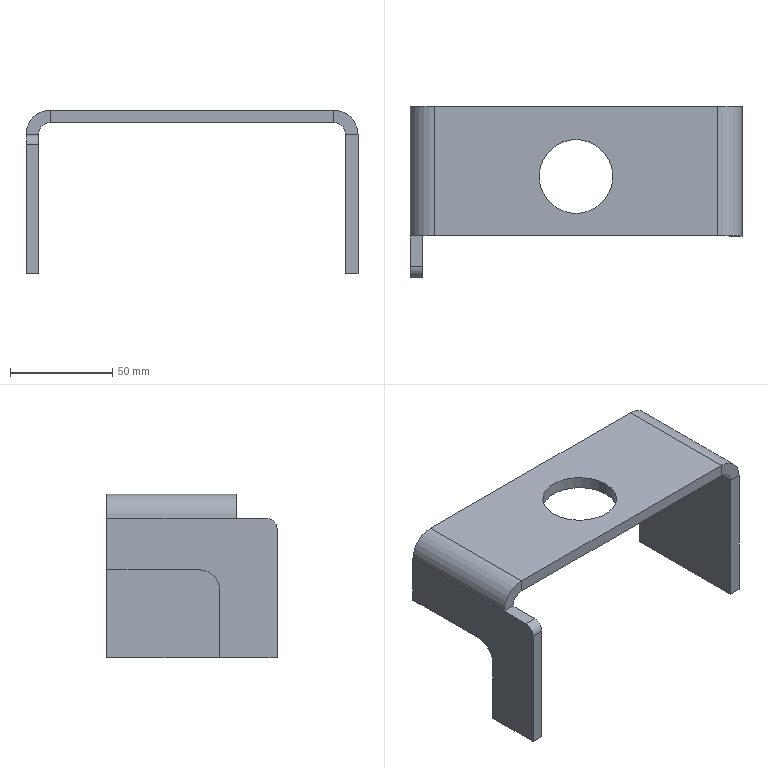Part | SolidWorks | features ICE 3, Fillet 2, FlatPattern 1, SMBaseFlange 1, SheetMetal 1 | 1 solid | 29 faces | box 162 x 83 x 80 mm | volume 102219 mm3 | plane 21 | cylinder 8 | commonest cylinder face diameters 12 x2 24 x2 36 x2 10 x1 20 x1
STEP:
#1=CARTESIAN_POINT('',(63.,49.,-6.));
#2=VERTEX_POINT('',#1);
#3=CARTESIAN_POINT('',(99.,49.,-6.));
#4=VERTEX_POINT('',#3);
#5=CARTESIAN_POINT('',(81.,49.,-6.));
#6=DIRECTION('',(0.,0.,1.));
#7=DIRECTION('',(1.,0.,0.));
#8=AXIS2_PLACEMENT_3D('',#5,#6,#7);
#9=CIRCLE('',#8,18.);
#10=EDGE_CURVE('',#2,#4,#9,.T.);
#11=ORIENTED_EDGE('',*,*,#10,.F.);
#12=CARTESIAN_POINT('',(63.,49.,0.));
#13=VERTEX_POINT('',#12);
#14=CARTESIAN_POINT('',(63.,49.,-6.));
#15=DIRECTION('',(0.,0.,1.));
#16=VECTOR('',#15,1000.);
#17=LINE('',#14,#16);
#18=EDGE_CURVE('',#2,#13,#17,.T.);
#19=ORIENTED_EDGE('',*,*,#18,.T.);
#20=CARTESIAN_POINT('',(99.,49.,0.));
#21=VERTEX_POINT('',#20);
#22=CARTESIAN_POINT('',(81.,49.,0.));
#23=DIRECTION('',(0.,0.,1.));
#24=DIRECTION('',(1.,0.,0.));
#25=AXIS2_PLACEMENT_3D('',#22,#23,#24);
#26=CIRCLE('',#25,18.);
#27=EDGE_CURVE('',#13,#21,#26,.T.);
#28=ORIENTED_EDGE('',*,*,#27,.T.);
#29=CARTESIAN_POINT('',(99.,49.,-6.));
#30=DIRECTION('',(0.,0.,1.));
#31=VECTOR('',#30,1000.);
#32=LINE('',#29,#31);
#33=EDGE_CURVE('',#4,#21,#32,.T.);
#34=ORIENTED_EDGE('',*,*,#33,.F.);
#35=EDGE_LOOP('',(#11,#19,#28,#34));
#36=FACE_OUTER_BOUND('',#35,.T.);
#37=CARTESIAN_POINT('',(81.,49.,-6.));
#38=DIRECTION('',(0.,0.,1.));
#39=DIRECTION('',(1.,0.,0.));
#40=AXIS2_PLACEMENT_3D('',#37,#38,#39);
#41=CYLINDRICAL_SURFACE('',#40,18.);
#42=ADVANCED_FACE('',(#36),#41,.F.);
#43=CARTESIAN_POINT('',(162.,20.,-12.));
#44=VERTEX_POINT('',#43);
#45=CARTESIAN_POINT('',(162.,20.,-80.));
#46=VERTEX_POINT('',#45);
#47=CARTESIAN_POINT('',(162.,20.,0.));
#48=DIRECTION('',(0.,0.,-1.));
#49=VECTOR('',#48,1000.);
#50=LINE('',#47,#49);
#51=EDGE_CURVE('',#44,#46,#50,.T.);
#52=ORIENTED_EDGE('',*,*,#51,.T.);
#53=CARTESIAN_POINT('',(162.,83.,-80.));
#54=VERTEX_POINT('',#53);
#55=CARTESIAN_POINT('',(162.,83.,-80.));
#56=DIRECTION('',(0.,-1.,0.));
#57=VECTOR('',#56,1000.);
#58=LINE('',#55,#57);
#59=EDGE_CURVE('',#54,#46,#58,.T.);
#60=ORIENTED_EDGE('',*,*,#59,.F.);
#61=CARTESIAN_POINT('',(162.,83.,-12.));
#62=VERTEX_POINT('',#61);
#63=CARTESIAN_POINT('',(162.,83.,0.));
#64=DIRECTION('',(0.,0.,-1.));
#65=VECTOR('',#64,1000.);
#66=LINE('',#63,#65);
#67=EDGE_CURVE('',#62,#54,#66,.T.);
#68=ORIENTED_EDGE('',*,*,#67,.F.);
#69=CARTESIAN_POINT('',(162.,83.,-12.));
#70=DIRECTION('',(0.,-1.,0.));
#71=VECTOR('',#70,1000.);
#72=LINE('',#69,#71);
#73=EDGE_CURVE('',#62,#44,#72,.T.);
#74=ORIENTED_EDGE('',*,*,#73,.T.);
#75=EDGE_LOOP('',(#52,#60,#68,#74));
#76=FACE_OUTER_BOUND('',#75,.T.);
#77=CARTESIAN_POINT('',(162.,83.,0.));
#78=DIRECTION('',(-1.,0.,0.));
#79=DIRECTION('',(0.,0.,1.));
#80=AXIS2_PLACEMENT_3D('',#77,#78,#79);
#81=PLANE('',#80);
#82=ADVANCED_FACE('',(#76),#81,.F.);
#83=ORIENTED_EDGE('',*,*,#59,.T.);
#84=CARTESIAN_POINT('',(156.,20.,-80.));
#85=VERTEX_POINT('',#84);
#86=CARTESIAN_POINT('',(156.,20.,-80.));
#87=DIRECTION('',(1.,0.,0.));
#88=VECTOR('',#87,1000.);
#89=LINE('',#86,#88);
#90=EDGE_CURVE('',#85,#46,#89,.T.);
#91=ORIENTED_EDGE('',*,*,#90,.F.);
#92=CARTESIAN_POINT('',(156.,83.,-80.));
#93=VERTEX_POINT('',#92);
#94=CARTESIAN_POINT('',(156.,83.,-80.));
#95=DIRECTION('',(0.,-1.,0.));
#96=VECTOR('',#95,1000.);
#97=LINE('',#94,#96);
#98=EDGE_CURVE('',#93,#85,#97,.T.);
#99=ORIENTED_EDGE('',*,*,#98,.F.);
#100=CARTESIAN_POINT('',(156.,83.,-80.));
#101=DIRECTION('',(1.,0.,0.));
#102=VECTOR('',#101,1000.);
#103=LINE('',#100,#102);
#104=EDGE_CURVE('',#93,#54,#103,.T.);
#105=ORIENTED_EDGE('',*,*,#104,.T.);
#106=EDGE_LOOP('',(#83,#91,#99,#105));
#107=FACE_OUTER_BOUND('',#106,.T.);
#108=CARTESIAN_POINT('',(156.,83.,-80.));
#109=DIRECTION('',(0.,0.,-1.));
#110=DIRECTION('',(-1.,0.,0.));
#111=AXIS2_PLACEMENT_3D('',#108,#109,#110);
#112=PLANE('',#111);
#113=ADVANCED_FACE('',(#107),#112,.T.);
#114=ORIENTED_EDGE('',*,*,#98,.T.);
#115=CARTESIAN_POINT('',(156.,20.,-12.));
#116=VERTEX_POINT('',#115);
#117=CARTESIAN_POINT('',(156.,20.,0.));
#118=DIRECTION('',(0.,0.,-1.));
#119=VECTOR('',#118,1000.);
#120=LINE('',#117,#119);
#121=EDGE_CURVE('',#116,#85,#120,.T.);
#122=ORIENTED_EDGE('',*,*,#121,.F.);
#123=CARTESIAN_POINT('',(156.,83.,-12.));
#124=VERTEX_POINT('',#123);
#125=CARTESIAN_POINT('',(156.,83.,-12.));
#126=DIRECTION('',(0.,-1.,0.));
#127=VECTOR('',#126,1000.);
#128=LINE('',#125,#127);
#129=EDGE_CURVE('',#124,#116,#128,.T.);
#130=ORIENTED_EDGE('',*,*,#129,.F.);
#131=CARTESIAN_POINT('',(156.,83.,0.));
#132=DIRECTION('',(0.,0.,-1.));
#133=VECTOR('',#132,1000.);
#134=LINE('',#131,#133);
#135=EDGE_CURVE('',#124,#93,#134,.T.);
#136=ORIENTED_EDGE('',*,*,#135,.T.);
#137=EDGE_LOOP('',(#114,#122,#130,#136));
#138=FACE_OUTER_BOUND('',#137,.T.);
#139=CARTESIAN_POINT('',(156.,83.,0.));
#140=DIRECTION('',(-1.,0.,0.));
#141=DIRECTION('',(0.,0.,1.));
#142=AXIS2_PLACEMENT_3D('',#139,#140,#141);
#143=PLANE('',#142);
#144=ADVANCED_FACE('',(#138),#143,.T.);
#145=ORIENTED_EDGE('',*,*,#129,.T.);
#146=CARTESIAN_POINT('',(150.,20.,-6.));
#147=VERTEX_POINT('',#146);
#148=CARTESIAN_POINT('',(150.,20.,-12.));
#149=DIRECTION('',(0.,1.,0.));
#150=DIRECTION('',(0.,0.,1.));
#151=AXIS2_PLACEMENT_3D('',#148,#149,#150);
#152=CIRCLE('',#151,6.);
#153=EDGE_CURVE('',#147,#116,#152,.T.);
#154=ORIENTED_EDGE('',*,*,#153,.F.);
#155=CARTESIAN_POINT('',(150.,83.,-6.));
#156=VERTEX_POINT('',#155);
#157=CARTESIAN_POINT('',(150.,83.,-6.));
#158=DIRECTION('',(0.,-1.,0.));
#159=VECTOR('',#158,1000.);
#160=LINE('',#157,#159);
#161=EDGE_CURVE('',#156,#147,#160,.T.);
#162=ORIENTED_EDGE('',*,*,#161,.F.);
#163=CARTESIAN_POINT('',(150.,83.,-12.));
#164=DIRECTION('',(0.,1.,0.));
#165=DIRECTION('',(1.,0.,0.));
#166=AXIS2_PLACEMENT_3D('',#163,#164,#165);
#167=CIRCLE('',#166,6.);
#168=EDGE_CURVE('',#156,#124,#167,.T.);
#169=ORIENTED_EDGE('',*,*,#168,.T.);
#170=EDGE_LOOP('',(#145,#154,#162,#169));
#171=FACE_OUTER_BOUND('',#170,.T.);
#172=CARTESIAN_POINT('',(150.,83.,-12.));
#173=DIRECTION('',(0.,-1.,0.));
#174=DIRECTION('',(0.,0.,-1.));
#175=AXIS2_PLACEMENT_3D('',#172,#173,#174);
#176=CYLINDRICAL_SURFACE('',#175,6.);
#177=ADVANCED_FACE('',(#171),#176,.F.);
#178=CARTESIAN_POINT('',(81.,49.,-6.));
#179=DIRECTION('',(0.,0.,1.));
#180=DIRECTION('',(1.,0.,0.));
#181=AXIS2_PLACEMENT_3D('',#178,#179,#180);
#182=CIRCLE('',#181,18.);
#183=EDGE_CURVE('',#4,#2,#182,.T.);
#184=ORIENTED_EDGE('',*,*,#183,.T.);
#185=ORIENTED_EDGE('',*,*,#10,.T.);
#186=EDGE_LOOP('',(#184,#185));
#187=FACE_BOUND('',#186,.T.);
#188=ORIENTED_EDGE('',*,*,#161,.T.);
#189=CARTESIAN_POINT('',(12.,20.,-6.));
#190=VERTEX_POINT('',#189);
#191=CARTESIAN_POINT('',(0.,20.,-6.));
#192=DIRECTION('',(1.,0.,0.));
#193=VECTOR('',#192,1000.);
#194=LINE('',#191,#193);
#195=EDGE_CURVE('',#190,#147,#194,.T.);
#196=ORIENTED_EDGE('',*,*,#195,.F.);
#197=CARTESIAN_POINT('',(12.,83.,-6.));
#198=VERTEX_POINT('',#197);
#199=CARTESIAN_POINT('',(12.,83.,-6.));
#200=DIRECTION('',(0.,-1.,0.));
#201=VECTOR('',#200,1000.);
#202=LINE('',#199,#201);
#203=EDGE_CURVE('',#198,#190,#202,.T.);
#204=ORIENTED_EDGE('',*,*,#203,.F.);
#205=CARTESIAN_POINT('',(0.,83.,-6.));
#206=DIRECTION('',(1.,0.,0.));
#207=VECTOR('',#206,1000.);
#208=LINE('',#205,#207);
#209=EDGE_CURVE('',#198,#156,#208,.T.);
#210=ORIENTED_EDGE('',*,*,#209,.T.);
#211=EDGE_LOOP('',(#188,#196,#204,#210));
#212=FACE_OUTER_BOUND('',#211,.T.);
#213=CARTESIAN_POINT('',(0.,83.,-6.));
#214=DIRECTION('',(0.,0.,-1.));
#215=DIRECTION('',(-1.,0.,0.));
#216=AXIS2_PLACEMENT_3D('',#213,#214,#215);
#217=PLANE('',#216);
#218=ADVANCED_FACE('',(#187,#212),#217,.T.);
#219=ORIENTED_EDGE('',*,*,#203,.T.);
#220=CARTESIAN_POINT('',(6.,20.,-12.));
#221=VERTEX_POINT('',#220);
#222=CARTESIAN_POINT('',(12.,20.,-12.));
#223=DIRECTION('',(0.,1.,0.));
#224=DIRECTION('',(0.,0.,1.));
#225=AXIS2_PLACEMENT_3D('',#222,#223,#224);
#226=CIRCLE('',#225,6.);
#227=EDGE_CURVE('',#221,#190,#226,.T.);
#228=ORIENTED_EDGE('',*,*,#227,.F.);
#229=CARTESIAN_POINT('',(6.,83.,-12.));
#230=VERTEX_POINT('',#229);
#231=CARTESIAN_POINT('',(6.,83.,-12.));
#232=DIRECTION('',(0.,-1.,0.));
#233=VECTOR('',#232,1000.);
#234=LINE('',#231,#233);
#235=EDGE_CURVE('',#230,#221,#234,.T.);
#236=ORIENTED_EDGE('',*,*,#235,.F.);
#237=CARTESIAN_POINT('',(12.,83.,-12.));
#238=DIRECTION('',(0.,1.,0.));
#239=DIRECTION('',(1.,0.,0.));
#240=AXIS2_PLACEMENT_3D('',#237,#238,#239);
#241=CIRCLE('',#240,6.);
#242=EDGE_CURVE('',#230,#198,#241,.T.);
#243=ORIENTED_EDGE('',*,*,#242,.T.);
#244=EDGE_LOOP('',(#219,#228,#236,#243));
#245=FACE_OUTER_BOUND('',#244,.T.);
#246=CARTESIAN_POINT('',(12.,83.,-12.));
#247=DIRECTION('',(0.,-1.,0.));
#248=DIRECTION('',(0.,0.,-1.));
#249=AXIS2_PLACEMENT_3D('',#246,#247,#248);
#250=CYLINDRICAL_SURFACE('',#249,6.);
#251=ADVANCED_FACE('',(#245),#250,.F.);
#252=CARTESIAN_POINT('',(0.,20.,-12.));
#253=VERTEX_POINT('',#252);
#254=CARTESIAN_POINT('',(12.,20.,0.));
#255=VERTEX_POINT('',#254);
#256=CARTESIAN_POINT('',(12.,20.,-12.));
#257=DIRECTION('',(0.,1.,0.));
#258=DIRECTION('',(0.,0.,-1.));
#259=AXIS2_PLACEMENT_3D('',#256,#257,#258);
#260=CIRCLE('',#259,12.);
#261=EDGE_CURVE('',#253,#255,#260,.T.);
#262=ORIENTED_EDGE('',*,*,#261,.T.);
#263=CARTESIAN_POINT('',(12.,83.,0.));
#264=VERTEX_POINT('',#263);
#265=CARTESIAN_POINT('',(12.,83.,0.));
#266=DIRECTION('',(0.,-1.,0.));
#267=VECTOR('',#266,1000.);
#268=LINE('',#265,#267);
#269=EDGE_CURVE('',#264,#255,#268,.T.);
#270=ORIENTED_EDGE('',*,*,#269,.F.);
#271=CARTESIAN_POINT('',(0.,83.,-12.));
#272=VERTEX_POINT('',#271);
#273=CARTESIAN_POINT('',(12.,83.,-12.));
#274=DIRECTION('',(0.,1.,0.));
#275=DIRECTION('',(0.,0.,-1.));
#276=AXIS2_PLACEMENT_3D('',#273,#274,#275);
#277=CIRCLE('',#276,12.);
#278=EDGE_CURVE('',#272,#264,#277,.T.);
#279=ORIENTED_EDGE('',*,*,#278,.F.);
#280=CARTESIAN_POINT('',(0.,83.,-12.));
#281=DIRECTION('',(0.,-1.,0.));
#282=VECTOR('',#281,1000.);
#283=LINE('',#280,#282);
#284=EDGE_CURVE('',#272,#253,#283,.T.);
#285=ORIENTED_EDGE('',*,*,#284,.T.);
#286=EDGE_LOOP('',(#262,#270,#279,#285));
#287=FACE_OUTER_BOUND('',#286,.T.);
#288=CARTESIAN_POINT('',(12.,83.,-12.));
#289=DIRECTION('',(0.,-1.,0.));
#290=DIRECTION('',(0.,0.,-1.));
#291=AXIS2_PLACEMENT_3D('',#288,#289,#290);
#292=CYLINDRICAL_SURFACE('',#291,12.);
#293=ADVANCED_FACE('',(#287),#292,.T.);
#294=CARTESIAN_POINT('',(81.,49.,0.));
#295=DIRECTION('',(0.,0.,1.));
#296=DIRECTION('',(1.,0.,0.));
#297=AXIS2_PLACEMENT_3D('',#294,#295,#296);
#298=CIRCLE('',#297,18.);
#299=EDGE_CURVE('',#21,#13,#298,.T.);
#300=ORIENTED_EDGE('',*,*,#299,.F.);
#301=ORIENTED_EDGE('',*,*,#27,.F.);
#302=EDGE_LOOP('',(#300,#301));
#303=FACE_BOUND('',#302,.T.);
#304=CARTESIAN_POINT('',(150.,20.,0.));
#305=VERTEX_POINT('',#304);
#306=CARTESIAN_POINT('',(0.,20.,0.));
#307=DIRECTION('',(1.,0.,0.));
#308=VECTOR('',#307,1000.);
#309=LINE('',#306,#308);
#310=EDGE_CURVE('',#255,#305,#309,.T.);
#311=ORIENTED_EDGE('',*,*,#310,.T.);
#312=CARTESIAN_POINT('',(150.,83.,0.));
#313=VERTEX_POINT('',#312);
#314=CARTESIAN_POINT('',(150.,83.,0.));
#315=DIRECTION('',(0.,-1.,0.));
#316=VECTOR('',#315,1000.);
#317=LINE('',#314,#316);
#318=EDGE_CURVE('',#313,#305,#317,.T.);
#319=ORIENTED_EDGE('',*,*,#318,.F.);
#320=CARTESIAN_POINT('',(0.,83.,0.));
#321=DIRECTION('',(1.,0.,0.));
#322=VECTOR('',#321,1000.);
#323=LINE('',#320,#322);
#324=EDGE_CURVE('',#264,#313,#323,.T.);
#325=ORIENTED_EDGE('',*,*,#324,.F.);
#326=ORIENTED_EDGE('',*,*,#269,.T.);
#327=EDGE_LOOP('',(#311,#319,#325,#326));
#328=FACE_OUTER_BOUND('',#327,.T.);
#329=CARTESIAN_POINT('',(0.,83.,0.));
#330=DIRECTION('',(0.,0.,-1.));
#331=DIRECTION('',(-1.,0.,0.));
#332=AXIS2_PLACEMENT_3D('',#329,#330,#331);
#333=PLANE('',#332);
#334=ADVANCED_FACE('',(#303,#328),#333,.F.);
#335=CARTESIAN_POINT('',(150.,20.,-12.));
#336=DIRECTION('',(0.,1.,0.));
#337=DIRECTION('',(0.,0.,-1.));
#338=AXIS2_PLACEMENT_3D('',#335,#336,#337);
#339=CIRCLE('',#338,12.);
#340=EDGE_CURVE('',#305,#44,#339,.T.);
#341=ORIENTED_EDGE('',*,*,#340,.T.);
#342=ORIENTED_EDGE('',*,*,#73,.F.);
#343=CARTESIAN_POINT('',(150.,83.,-12.));
#344=DIRECTION('',(0.,1.,0.));
#345=DIRECTION('',(0.,0.,-1.));
#346=AXIS2_PLACEMENT_3D('',#343,#344,#345);
#347=CIRCLE('',#346,12.);
#348=EDGE_CURVE('',#313,#62,#347,.T.);
#349=ORIENTED_EDGE('',*,*,#348,.F.);
#350=ORIENTED_EDGE('',*,*,#318,.T.);
#351=EDGE_LOOP('',(#341,#342,#349,#350));
#352=FACE_OUTER_BOUND('',#351,.T.);
#353=CARTESIAN_POINT('',(150.,83.,-12.));
#354=DIRECTION('',(0.,-1.,0.));
#355=DIRECTION('',(0.,0.,-1.));
#356=AXIS2_PLACEMENT_3D('',#353,#354,#355);
#357=CYLINDRICAL_SURFACE('',#356,12.);
#358=ADVANCED_FACE('',(#352),#357,.T.);
#359=CARTESIAN_POINT('',(0.,83.,-12.));
#360=DIRECTION('',(1.,0.,0.));
#361=VECTOR('',#360,1000.);
#362=LINE('',#359,#361);
#363=EDGE_CURVE('',#272,#230,#362,.T.);
#364=ORIENTED_EDGE('',*,*,#363,.F.);
#365=ORIENTED_EDGE('',*,*,#278,.T.);
#366=CARTESIAN_POINT('',(12.,83.,-6.));
#367=DIRECTION('',(0.,0.,1.));
#368=VECTOR('',#367,1000.);
#369=LINE('',#366,#368);
#370=EDGE_CURVE('',#198,#264,#369,.T.);
#371=ORIENTED_EDGE('',*,*,#370,.F.);
#372=ORIENTED_EDGE('',*,*,#242,.F.);
#373=EDGE_LOOP('',(#364,#365,#371,#372));
#374=FACE_OUTER_BOUND('',#373,.T.);
#375=CARTESIAN_POINT('',(0.,83.,-12.));
#376=DIRECTION('',(0.,1.,0.));
#377=DIRECTION('',(0.,0.,1.));
#378=AXIS2_PLACEMENT_3D('',#375,#376,#377);
#379=PLANE('',#378);
#380=ADVANCED_FACE('',(#374),#379,.T.);
#381=CARTESIAN_POINT('',(6.,83.,-37.));
#382=VERTEX_POINT('',#381);
#383=CARTESIAN_POINT('',(0.,83.,-37.));
#384=VERTEX_POINT('',#383);
#385=CARTESIAN_POINT('',(6.,83.,-37.));
#386=DIRECTION('',(-1.,0.,0.));
#387=VECTOR('',#386,1000.);
#388=LINE('',#385,#387);
#389=EDGE_CURVE('',#382,#384,#388,.T.);
#390=ORIENTED_EDGE('',*,*,#389,.T.);
#391=CARTESIAN_POINT('',(0.,83.,-80.));
#392=DIRECTION('',(0.,0.,1.));
#393=VECTOR('',#392,1000.);
#394=LINE('',#391,#393);
#395=EDGE_CURVE('',#384,#272,#394,.T.);
#396=ORIENTED_EDGE('',*,*,#395,.T.);
#397=ORIENTED_EDGE('',*,*,#363,.T.);
#398=CARTESIAN_POINT('',(6.,83.,-80.));
#399=DIRECTION('',(0.,0.,1.));
#400=VECTOR('',#399,1000.);
#401=LINE('',#398,#400);
#402=EDGE_CURVE('',#382,#230,#401,.T.);
#403=ORIENTED_EDGE('',*,*,#402,.F.);
#404=EDGE_LOOP('',(#390,#396,#397,#403));
#405=FACE_OUTER_BOUND('',#404,.T.);
#406=CARTESIAN_POINT('',(12.,83.,-6.));
#407=DIRECTION('',(0.,1.,0.));
#408=DIRECTION('',(0.,0.,1.));
#409=AXIS2_PLACEMENT_3D('',#406,#407,#408);
#410=PLANE('',#409);
#411=ADVANCED_FACE('',(#405),#410,.T.);
#412=CARTESIAN_POINT('',(150.,83.,0.));
#413=DIRECTION('',(0.,0.,-1.));
#414=VECTOR('',#413,1000.);
#415=LINE('',#412,#414);
#416=EDGE_CURVE('',#313,#156,#415,.T.);
#417=ORIENTED_EDGE('',*,*,#416,.F.);
#418=ORIENTED_EDGE('',*,*,#348,.T.);
#419=CARTESIAN_POINT('',(156.,83.,-12.));
#420=DIRECTION('',(1.,0.,0.));
#421=VECTOR('',#420,1000.);
#422=LINE('',#419,#421);
#423=EDGE_CURVE('',#124,#62,#422,.T.);
#424=ORIENTED_EDGE('',*,*,#423,.F.);
#425=ORIENTED_EDGE('',*,*,#168,.F.);
#426=EDGE_LOOP('',(#417,#418,#424,#425));
#427=FACE_OUTER_BOUND('',#426,.T.);
#428=CARTESIAN_POINT('',(150.,83.,0.));
#429=DIRECTION('',(0.,1.,0.));
#430=DIRECTION('',(0.,0.,1.));
#431=AXIS2_PLACEMENT_3D('',#428,#429,#430);
#432=PLANE('',#431);
#433=ADVANCED_FACE('',(#427),#432,.T.);
#434=ORIENTED_EDGE('',*,*,#324,.T.);
#435=ORIENTED_EDGE('',*,*,#416,.T.);
#436=ORIENTED_EDGE('',*,*,#209,.F.);
#437=ORIENTED_EDGE('',*,*,#370,.T.);
#438=EDGE_LOOP('',(#434,#435,#436,#437));
#439=FACE_OUTER_BOUND('',#438,.T.);
#440=CARTESIAN_POINT('',(156.,83.,-12.));
#441=DIRECTION('',(0.,1.,0.));
#442=DIRECTION('',(0.,0.,1.));
#443=AXIS2_PLACEMENT_3D('',#440,#441,#442);
#444=PLANE('',#443);
#445=ADVANCED_FACE('',(#439),#444,.T.);
#446=CARTESIAN_POINT('',(6.,5.,-12.));
#447=VERTEX_POINT('',#446);
#448=CARTESIAN_POINT('',(6.,83.,-12.));
#449=DIRECTION('',(0.,-1.,0.));
#450=VECTOR('',#449,1000.);
#451=LINE('',#448,#450);
#452=EDGE_CURVE('',#221,#447,#451,.T.);
#453=ORIENTED_EDGE('',*,*,#452,.T.);
#454=CARTESIAN_POINT('',(6.,0.,-17.));
#455=VERTEX_POINT('',#454);
#456=CARTESIAN_POINT('',(6.,5.,-17.));
#457=DIRECTION('',(1.,0.,0.));
#458=DIRECTION('',(0.,0.,-1.));
#459=AXIS2_PLACEMENT_3D('',#456,#457,#458);
#460=CIRCLE('',#459,5.);
#461=EDGE_CURVE('',#447,#455,#460,.T.);
#462=ORIENTED_EDGE('',*,*,#461,.T.);
#463=CARTESIAN_POINT('',(6.,0.,-80.));
#464=VERTEX_POINT('',#463);
#465=CARTESIAN_POINT('',(6.,0.,-80.));
#466=DIRECTION('',(0.,0.,1.));
#467=VECTOR('',#466,1000.);
#468=LINE('',#465,#467);
#469=EDGE_CURVE('',#464,#455,#468,.T.);
#470=ORIENTED_EDGE('',*,*,#469,.F.);
#471=CARTESIAN_POINT('',(6.,28.,-80.));
#472=VERTEX_POINT('',#471);
#473=CARTESIAN_POINT('',(6.,83.,-80.));
#474=DIRECTION('',(0.,-1.,0.));
#475=VECTOR('',#474,1000.);
#476=LINE('',#473,#475);
#477=EDGE_CURVE('',#472,#464,#476,.T.);
#478=ORIENTED_EDGE('',*,*,#477,.F.);
#479=CARTESIAN_POINT('',(6.,28.,-47.));
#480=VERTEX_POINT('',#479);
#481=CARTESIAN_POINT('',(6.,28.,-80.));
#482=DIRECTION('',(0.,0.,1.));
#483=VECTOR('',#482,1000.);
#484=LINE('',#481,#483);
#485=EDGE_CURVE('',#472,#480,#484,.T.);
#486=ORIENTED_EDGE('',*,*,#485,.T.);
#487=CARTESIAN_POINT('',(6.,38.,-37.));
#488=VERTEX_POINT('',#487);
#489=CARTESIAN_POINT('',(6.,38.,-47.));
#490=DIRECTION('',(-1.,0.,0.));
#491=DIRECTION('',(0.,0.,-1.));
#492=AXIS2_PLACEMENT_3D('',#489,#490,#491);
#493=CIRCLE('',#492,10.);
#494=EDGE_CURVE('',#480,#488,#493,.T.);
#495=ORIENTED_EDGE('',*,*,#494,.T.);
#496=CARTESIAN_POINT('',(6.,83.,-37.));
#497=DIRECTION('',(0.,1.,0.));
#498=VECTOR('',#497,1000.);
#499=LINE('',#496,#498);
#500=EDGE_CURVE('',#488,#382,#499,.T.);
#501=ORIENTED_EDGE('',*,*,#500,.T.);
#502=ORIENTED_EDGE('',*,*,#402,.T.);
#503=ORIENTED_EDGE('',*,*,#235,.T.);
#504=EDGE_LOOP('',(#453,#462,#470,#478,#486,#495,#501,#502,#503));
#505=FACE_OUTER_BOUND('',#504,.T.);
#506=CARTESIAN_POINT('',(6.,83.,-80.));
#507=DIRECTION('',(1.,0.,0.));
#508=DIRECTION('',(0.,0.,-1.));
#509=AXIS2_PLACEMENT_3D('',#506,#507,#508);
#510=PLANE('',#509);
#511=ADVANCED_FACE('',(#505),#510,.T.);
#512=CARTESIAN_POINT('',(0.,28.,-80.));
#513=VERTEX_POINT('',#512);
#514=CARTESIAN_POINT('',(6.,28.,-80.));
#515=DIRECTION('',(-1.,0.,0.));
#516=VECTOR('',#515,1000.);
#517=LINE('',#514,#516);
#518=EDGE_CURVE('',#472,#513,#517,.T.);
#519=ORIENTED_EDGE('',*,*,#518,.F.);
#520=ORIENTED_EDGE('',*,*,#477,.T.);
#521=CARTESIAN_POINT('',(0.,0.,-80.));
#522=VERTEX_POINT('',#521);
#523=CARTESIAN_POINT('',(0.,0.,-80.));
#524=DIRECTION('',(1.,0.,0.));
#525=VECTOR('',#524,1000.);
#526=LINE('',#523,#525);
#527=EDGE_CURVE('',#522,#464,#526,.T.);
#528=ORIENTED_EDGE('',*,*,#527,.F.);
#529=CARTESIAN_POINT('',(0.,83.,-80.));
#530=DIRECTION('',(0.,-1.,0.));
#531=VECTOR('',#530,1000.);
#532=LINE('',#529,#531);
#533=EDGE_CURVE('',#513,#522,#532,.T.);
#534=ORIENTED_EDGE('',*,*,#533,.F.);
#535=EDGE_LOOP('',(#519,#520,#528,#534));
#536=FACE_OUTER_BOUND('',#535,.T.);
#537=CARTESIAN_POINT('',(0.,83.,-80.));
#538=DIRECTION('',(0.,0.,-1.));
#539=DIRECTION('',(-1.,0.,0.));
#540=AXIS2_PLACEMENT_3D('',#537,#538,#539);
#541=PLANE('',#540);
#542=ADVANCED_FACE('',(#536),#541,.T.);
#543=CARTESIAN_POINT('',(0.,0.,-17.));
#544=VERTEX_POINT('',#543);
#545=CARTESIAN_POINT('',(0.,0.,-80.));
#546=DIRECTION('',(0.,0.,1.));
#547=VECTOR('',#546,1000.);
#548=LINE('',#545,#547);
#549=EDGE_CURVE('',#522,#544,#548,.T.);
#550=ORIENTED_EDGE('',*,*,#549,.T.);
#551=CARTESIAN_POINT('',(0.,5.,-12.));
#552=VERTEX_POINT('',#551);
#553=CARTESIAN_POINT('',(0.,5.,-17.));
#554=DIRECTION('',(-1.,0.,0.));
#555=DIRECTION('',(0.,0.,-1.));
#556=AXIS2_PLACEMENT_3D('',#553,#554,#555);
#557=CIRCLE('',#556,5.);
#558=EDGE_CURVE('',#544,#552,#557,.T.);
#559=ORIENTED_EDGE('',*,*,#558,.T.);
#560=CARTESIAN_POINT('',(0.,83.,-12.));
#561=DIRECTION('',(0.,-1.,0.));
#562=VECTOR('',#561,1000.);
#563=LINE('',#560,#562);
#564=EDGE_CURVE('',#253,#552,#563,.T.);
#565=ORIENTED_EDGE('',*,*,#564,.F.);
#566=ORIENTED_EDGE('',*,*,#284,.F.);
#567=ORIENTED_EDGE('',*,*,#395,.F.);
#568=CARTESIAN_POINT('',(0.,38.,-37.));
#569=VERTEX_POINT('',#568);
#570=CARTESIAN_POINT('',(0.,83.,-37.));
#571=DIRECTION('',(0.,1.,0.));
#572=VECTOR('',#571,1000.);
#573=LINE('',#570,#572);
#574=EDGE_CURVE('',#569,#384,#573,.T.);
#575=ORIENTED_EDGE('',*,*,#574,.F.);
#576=CARTESIAN_POINT('',(0.,28.,-47.));
#577=VERTEX_POINT('',#576);
#578=CARTESIAN_POINT('',(0.,38.,-47.));
#579=DIRECTION('',(1.,0.,0.));
#580=DIRECTION('',(0.,0.,-1.));
#581=AXIS2_PLACEMENT_3D('',#578,#579,#580);
#582=CIRCLE('',#581,10.);
#583=EDGE_CURVE('',#569,#577,#582,.T.);
#584=ORIENTED_EDGE('',*,*,#583,.T.);
#585=CARTESIAN_POINT('',(0.,28.,-80.));
#586=DIRECTION('',(0.,0.,1.));
#587=VECTOR('',#586,1000.);
#588=LINE('',#585,#587);
#589=EDGE_CURVE('',#513,#577,#588,.T.);
#590=ORIENTED_EDGE('',*,*,#589,.F.);
#591=ORIENTED_EDGE('',*,*,#533,.T.);
#592=EDGE_LOOP('',(#550,#559,#565,#566,#567,#575,#584,#590,#591));
#593=FACE_OUTER_BOUND('',#592,.T.);
#594=CARTESIAN_POINT('',(0.,83.,-80.));
#595=DIRECTION('',(1.,0.,0.));
#596=DIRECTION('',(0.,0.,-1.));
#597=AXIS2_PLACEMENT_3D('',#594,#595,#596);
#598=PLANE('',#597);
#599=ADVANCED_FACE('',(#593),#598,.F.);
#600=ORIENTED_EDGE('',*,*,#67,.T.);
#601=ORIENTED_EDGE('',*,*,#104,.F.);
#602=ORIENTED_EDGE('',*,*,#135,.F.);
#603=ORIENTED_EDGE('',*,*,#423,.T.);
#604=EDGE_LOOP('',(#600,#601,#602,#603));
#605=FACE_OUTER_BOUND('',#604,.T.);
#606=CARTESIAN_POINT('',(150.,83.,-12.));
#607=DIRECTION('',(0.,1.,0.));
#608=DIRECTION('',(1.,0.,0.));
#609=AXIS2_PLACEMENT_3D('',#606,#607,#608);
#610=PLANE('',#609);
#611=ADVANCED_FACE('',(#605),#610,.T.);
#612=ORIENTED_EDGE('',*,*,#469,.T.);
#613=CARTESIAN_POINT('',(0.,0.,-17.));
#614=DIRECTION('',(-1.,0.,0.));
#615=VECTOR('',#614,1000.);
#616=LINE('',#613,#615);
#617=EDGE_CURVE('',#455,#544,#616,.T.);
#618=ORIENTED_EDGE('',*,*,#617,.T.);
#619=ORIENTED_EDGE('',*,*,#549,.F.);
#620=ORIENTED_EDGE('',*,*,#527,.T.);
#621=EDGE_LOOP('',(#612,#618,#619,#620));
#622=FACE_OUTER_BOUND('',#621,.T.);
#623=CARTESIAN_POINT('',(150.,0.,-12.));
#624=DIRECTION('',(0.,1.,0.));
#625=DIRECTION('',(1.,0.,0.));
#626=AXIS2_PLACEMENT_3D('',#623,#624,#625);
#627=PLANE('',#626);
#628=ADVANCED_FACE('',(#622),#627,.F.);
#629=ORIENTED_EDGE('',*,*,#121,.T.);
#630=ORIENTED_EDGE('',*,*,#90,.T.);
#631=ORIENTED_EDGE('',*,*,#51,.F.);
#632=CARTESIAN_POINT('',(156.,20.,-12.));
#633=DIRECTION('',(1.,0.,0.));
#634=VECTOR('',#633,1000.);
#635=LINE('',#632,#634);
#636=EDGE_CURVE('',#116,#44,#635,.T.);
#637=ORIENTED_EDGE('',*,*,#636,.F.);
#638=EDGE_LOOP('',(#629,#630,#631,#637));
#639=FACE_OUTER_BOUND('',#638,.T.);
#640=CARTESIAN_POINT('',(156.,20.,0.));
#641=DIRECTION('',(0.,1.,0.));
#642=DIRECTION('',(0.,0.,-1.));
#643=AXIS2_PLACEMENT_3D('',#640,#641,#642);
#644=PLANE('',#643);
#645=ADVANCED_FACE('',(#639),#644,.F.);
#646=ORIENTED_EDGE('',*,*,#195,.T.);
#647=CARTESIAN_POINT('',(150.,20.,-6.));
#648=DIRECTION('',(0.,0.,1.));
#649=VECTOR('',#648,1000.);
#650=LINE('',#647,#649);
#651=EDGE_CURVE('',#147,#305,#650,.T.);
#652=ORIENTED_EDGE('',*,*,#651,.T.);
#653=ORIENTED_EDGE('',*,*,#310,.F.);
#654=CARTESIAN_POINT('',(12.,20.,-6.));
#655=DIRECTION('',(0.,0.,1.));
#656=VECTOR('',#655,1000.);
#657=LINE('',#654,#656);
#658=EDGE_CURVE('',#190,#255,#657,.T.);
#659=ORIENTED_EDGE('',*,*,#658,.F.);
#660=EDGE_LOOP('',(#646,#652,#653,#659));
#661=FACE_OUTER_BOUND('',#660,.T.);
#662=CARTESIAN_POINT('',(0.,20.,-6.));
#663=DIRECTION('',(0.,1.,0.));
#664=DIRECTION('',(1.,0.,0.));
#665=AXIS2_PLACEMENT_3D('',#662,#663,#664);
#666=PLANE('',#665);
#667=ADVANCED_FACE('',(#661),#666,.F.);
#668=ORIENTED_EDGE('',*,*,#153,.T.);
#669=ORIENTED_EDGE('',*,*,#636,.T.);
#670=ORIENTED_EDGE('',*,*,#340,.F.);
#671=ORIENTED_EDGE('',*,*,#651,.F.);
#672=EDGE_LOOP('',(#668,#669,#670,#671));
#673=FACE_OUTER_BOUND('',#672,.T.);
#674=CARTESIAN_POINT('',(150.,20.,-12.));
#675=DIRECTION('',(0.,-1.,0.));
#676=DIRECTION('',(0.,0.,-1.));
#677=AXIS2_PLACEMENT_3D('',#674,#675,#676);
#678=PLANE('',#677);
#679=ADVANCED_FACE('',(#673),#678,.T.);
#680=ORIENTED_EDGE('',*,*,#564,.T.);
#681=CARTESIAN_POINT('',(6.,5.,-12.));
#682=DIRECTION('',(1.,0.,0.));
#683=VECTOR('',#682,1000.);
#684=LINE('',#681,#683);
#685=EDGE_CURVE('',#552,#447,#684,.T.);
#686=ORIENTED_EDGE('',*,*,#685,.T.);
#687=ORIENTED_EDGE('',*,*,#452,.F.);
#688=CARTESIAN_POINT('',(6.,20.,-12.));
#689=DIRECTION('',(-1.,0.,0.));
#690=VECTOR('',#689,1000.);
#691=LINE('',#688,#690);
#692=EDGE_CURVE('',#221,#253,#691,.T.);
#693=ORIENTED_EDGE('',*,*,#692,.T.);
#694=EDGE_LOOP('',(#680,#686,#687,#693));
#695=FACE_OUTER_BOUND('',#694,.T.);
#696=CARTESIAN_POINT('',(6.,10.,-12.));
#697=DIRECTION('',(0.,0.,-1.));
#698=DIRECTION('',(0.,-1.,0.));
#699=AXIS2_PLACEMENT_3D('',#696,#697,#698);
#700=PLANE('',#699);
#701=ADVANCED_FACE('',(#695),#700,.F.);
#702=ORIENTED_EDGE('',*,*,#658,.T.);
#703=ORIENTED_EDGE('',*,*,#261,.F.);
#704=ORIENTED_EDGE('',*,*,#692,.F.);
#705=ORIENTED_EDGE('',*,*,#227,.T.);
#706=EDGE_LOOP('',(#702,#703,#704,#705));
#707=FACE_OUTER_BOUND('',#706,.T.);
#708=CARTESIAN_POINT('',(12.,20.,-12.));
#709=DIRECTION('',(0.,-1.,0.));
#710=DIRECTION('',(0.,0.,-1.));
#711=AXIS2_PLACEMENT_3D('',#708,#709,#710);
#712=PLANE('',#711);
#713=ADVANCED_FACE('',(#707),#712,.T.);
#714=ORIENTED_EDGE('',*,*,#500,.F.);
#715=CARTESIAN_POINT('',(0.,38.,-37.));
#716=DIRECTION('',(-1.,0.,0.));
#717=VECTOR('',#716,1000.);
#718=LINE('',#715,#717);
#719=EDGE_CURVE('',#488,#569,#718,.T.);
#720=ORIENTED_EDGE('',*,*,#719,.T.);
#721=ORIENTED_EDGE('',*,*,#574,.T.);
#722=ORIENTED_EDGE('',*,*,#389,.F.);
#723=EDGE_LOOP('',(#714,#720,#721,#722));
#724=FACE_OUTER_BOUND('',#723,.T.);
#725=CARTESIAN_POINT('',(6.,83.,-37.));
#726=DIRECTION('',(0.,0.,1.));
#727=DIRECTION('',(0.,-1.,0.));
#728=AXIS2_PLACEMENT_3D('',#725,#726,#727);
#729=PLANE('',#728);
#730=ADVANCED_FACE('',(#724),#729,.F.);
#731=ORIENTED_EDGE('',*,*,#589,.T.);
#732=CARTESIAN_POINT('',(6.,28.,-47.));
#733=DIRECTION('',(1.,0.,0.));
#734=VECTOR('',#733,1000.);
#735=LINE('',#732,#734);
#736=EDGE_CURVE('',#577,#480,#735,.T.);
#737=ORIENTED_EDGE('',*,*,#736,.T.);
#738=ORIENTED_EDGE('',*,*,#485,.F.);
#739=ORIENTED_EDGE('',*,*,#518,.T.);
#740=EDGE_LOOP('',(#731,#737,#738,#739));
#741=FACE_OUTER_BOUND('',#740,.T.);
#742=CARTESIAN_POINT('',(6.,28.,-80.));
#743=DIRECTION('',(0.,-1.,0.));
#744=DIRECTION('',(0.,0.,-1.));
#745=AXIS2_PLACEMENT_3D('',#742,#743,#744);
#746=PLANE('',#745);
#747=ADVANCED_FACE('',(#741),#746,.F.);
#748=ORIENTED_EDGE('',*,*,#461,.F.);
#749=ORIENTED_EDGE('',*,*,#685,.F.);
#750=ORIENTED_EDGE('',*,*,#558,.F.);
#751=ORIENTED_EDGE('',*,*,#617,.F.);
#752=EDGE_LOOP('',(#748,#749,#750,#751));
#753=FACE_OUTER_BOUND('',#752,.T.);
#754=CARTESIAN_POINT('',(150.,5.,-17.));
#755=DIRECTION('',(-1.,0.,0.));
#756=DIRECTION('',(0.,0.,1.));
#757=AXIS2_PLACEMENT_3D('',#754,#755,#756);
#758=CYLINDRICAL_SURFACE('',#757,5.);
#759=ADVANCED_FACE('',(#753),#758,.T.);
#760=ORIENTED_EDGE('',*,*,#494,.F.);
#761=ORIENTED_EDGE('',*,*,#736,.F.);
#762=ORIENTED_EDGE('',*,*,#583,.F.);
#763=ORIENTED_EDGE('',*,*,#719,.F.);
#764=EDGE_LOOP('',(#760,#761,#762,#763));
#765=FACE_OUTER_BOUND('',#764,.T.);
#766=CARTESIAN_POINT('',(6.,38.,-47.));
#767=DIRECTION('',(1.,0.,0.));
#768=DIRECTION('',(0.,0.,-1.));
#769=AXIS2_PLACEMENT_3D('',#766,#767,#768);
#770=CYLINDRICAL_SURFACE('',#769,10.);
#771=ADVANCED_FACE('',(#765),#770,.F.);
#772=ORIENTED_EDGE('',*,*,#18,.F.);
#773=ORIENTED_EDGE('',*,*,#183,.F.);
#774=ORIENTED_EDGE('',*,*,#33,.T.);
#775=ORIENTED_EDGE('',*,*,#299,.T.);
#776=EDGE_LOOP('',(#772,#773,#774,#775));
#777=FACE_OUTER_BOUND('',#776,.T.);
#778=CARTESIAN_POINT('',(81.,49.,-6.));
#779=DIRECTION('',(0.,0.,1.));
#780=DIRECTION('',(1.,0.,0.));
#781=AXIS2_PLACEMENT_3D('',#778,#779,#780);
#782=CYLINDRICAL_SURFACE('',#781,18.);
#783=ADVANCED_FACE('',(#777),#782,.F.);
#784=CLOSED_SHELL('',(#42,#82,#113,#144,#177,#218,#251,#293,#334,#358,#380,#411,#433,#445,#511,#542,#599,#611,#628,#645,#667,#679,#701,#713,#730,#747,#759,#771,#783));
#785=MANIFOLD_SOLID_BREP('',#784);
#786=CARTESIAN_POINT('',(0.,0.,0.));
#787=DIRECTION('',(0.,0.,1.));
#788=DIRECTION('',(1.,0.,0.));
#789=AXIS2_PLACEMENT_3D('',#786,#787,#788);
#790=(LENGTH_UNIT()NAMED_UNIT(*)SI_UNIT(.MILLI.,.METRE.));
#791=UNCERTAINTY_MEASURE_WITH_UNIT(LENGTH_MEASURE(0.00001),#790,'','');
#792=(NAMED_UNIT(*)PLANE_ANGLE_UNIT()SI_UNIT($,.RADIAN.));
#793=(NAMED_UNIT(*)SI_UNIT($,.STERADIAN.)SOLID_ANGLE_UNIT());
#794=(GEOMETRIC_REPRESENTATION_CONTEXT(3)GLOBAL_UNCERTAINTY_ASSIGNED_CONTEXT((#791))GLOBAL_UNIT_ASSIGNED_CONTEXT((#790,#792,#793))REPRESENTATION_CONTEXT('',''));
#795=ADVANCED_BREP_SHAPE_REPRESENTATION('',(#785,#789),#794);